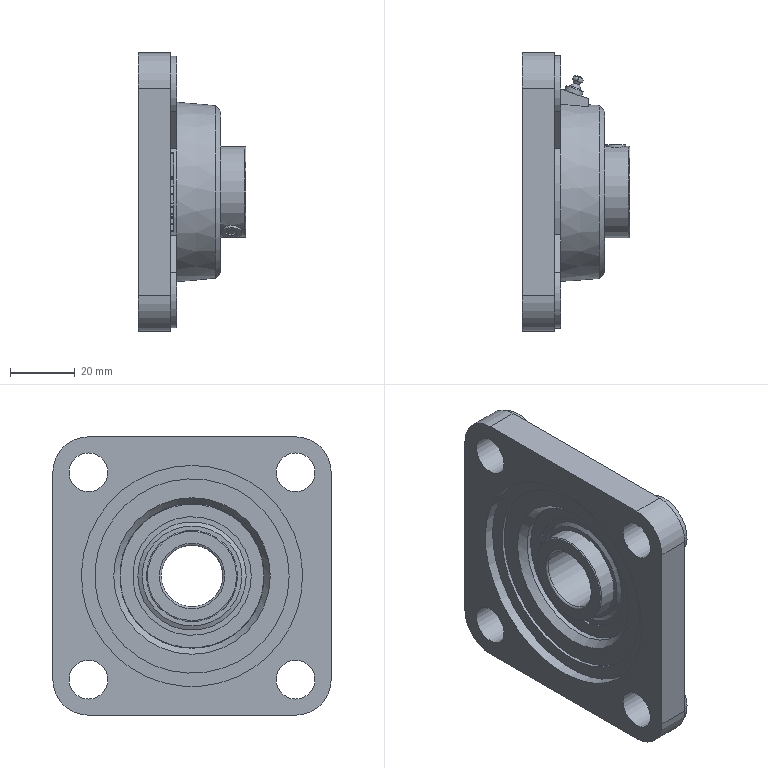Part | STEP file | FYJ_3_4_TF_2_14a | 10 solids | 244 faces | box 33.3 x 86 x 86 mm | volume 78576 mm3 | plane 115 | cylinder 95 | sphere 11 | cone 10 | torus 9 | other 4 | commonest cylinder face diameters 0.5 x54 28.2 x6 60.995 x5 12 x4 20 x4 22 x4